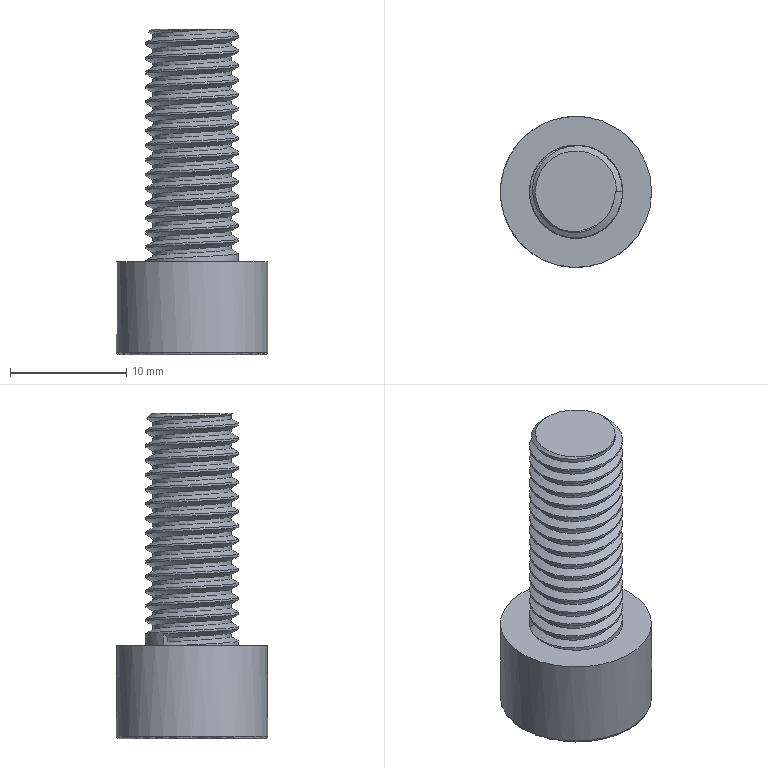Part | STEP file | Tube feed_id1458_x_t | 1 solid | 26 faces | box 13 x 13 x 28 mm | volume 1716 mm3 | plane 12 | cylinder 9 | spline 3 | cone 1 | torus 1 | commonest cylinder face diameters 0.4 x6 6.75 x1 8 x1 13 x1